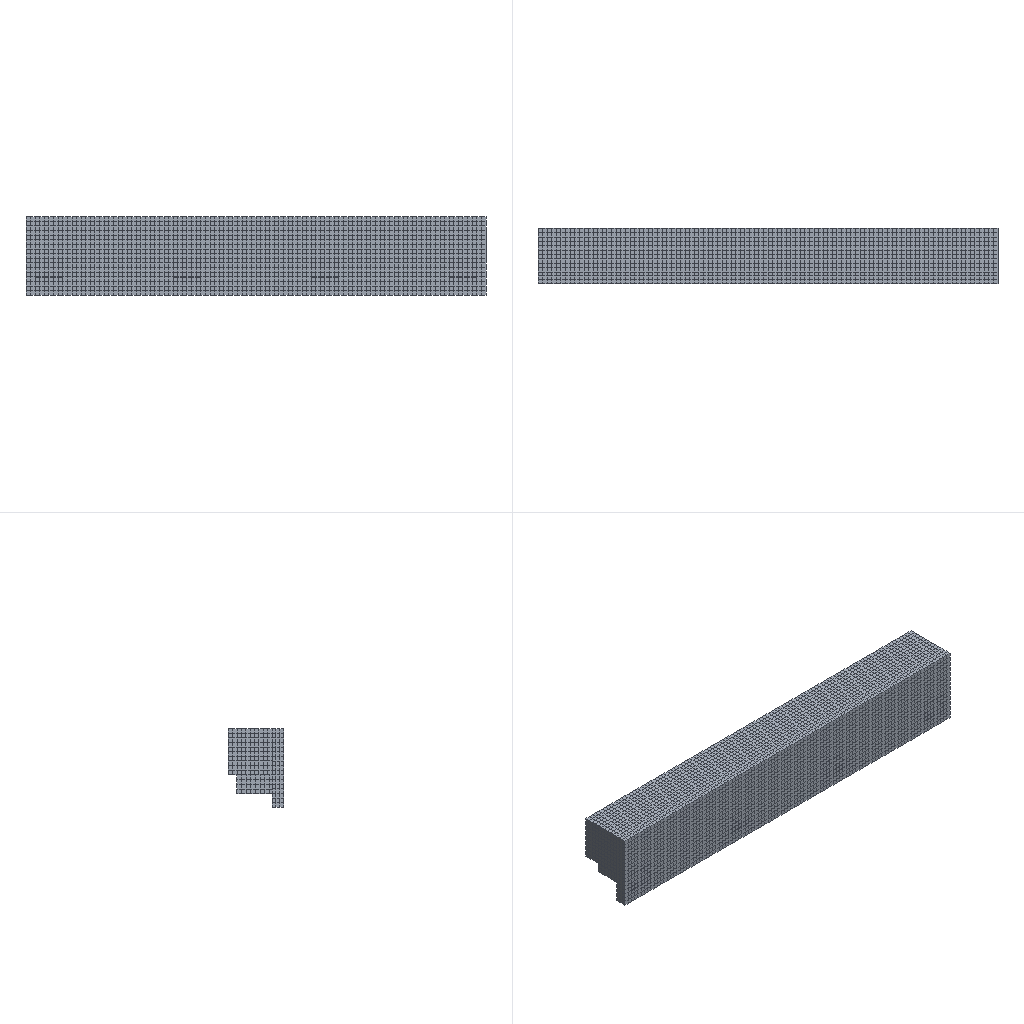Simulation study
Set-up summary:
category,name,step,type,value,unit,region
solver,abaqus
solver,version,,,Abaqus/Explicit 2020
units,not stated in the deck,,not stated
analysis,deck,,transient,transient
load_step,Step-1,Step-1,transient,nlgeom=True
contact,interactions,,,general=1 pairs=0 ties=0
load_step,requested,,,1
mesh,nodes,,,22863
mesh,elements,,,17308
element_type,C3D8R,,solid,17308
load,load commands in deck,,count,1
bc,support commands in deck,,count,6
material,MATERIAL-1,,in results
material,WATER,,in results
check,setup vs results,,match,"per instance, exact: element labels, types and connectivity; labels of the nodes the elements use; coordinates of those nodes at SINGLE_PRECISION in 3 of 3 instance(s)"
Abaqus input file, long lists of numbers shortened:
*Heading
** Job name: Job-1 Model name: Model-1
** Generated by: Abaqus/CAE 2020
*Preprint, echo=NO, model=NO, history=NO, contact=NO
**
** PARTS
**
*Part, name=Part-1
*Node
      1,           2.,           0.,           0.
      2,           4.,           0.,           0.
** (3368 more lines like these left out)
*Element, type=C3D8R
   1,   16,  299,  392,  157,  690,  973, 1066,  831
   2,  529,   95,  472,  502, 1203,  769, 1146, 1176
** (2206 more lines like these left out)
*Nset, nset=Set-1, generate
    1,  3370,     1
*Elset, elset=Set-1, generate
    1,  2208,     1
** Section: Section-1
*Solid Section, elset=Set-1, material=Material-1
,
*End Part
**
*Part, name=water-chong
*Node
      1,           0.,         -9.5,          10.
      2,           0.,  -8.55,          10.
** (12219 more lines like these left out)
*Element, type=C3D8R
    1,   122,   123,   134,   133,     1,     2,    13,    12
    2,   123,   124,   135,   134,     2,     3,    14,    13
** (9998 more lines like these left out)
*Nset, nset=Set-1, generate
     1,  12221,      1
*Elset, elset=Set-1, generate
     1,  10000,      1
** Section: water
*Solid Section, elset=Set-1, controls=EC-1, material=water
,
*End Part
**
*Part, name=water-original
*Node
      1,           0.,         -2.5,   17.1
      2,           0.,  -1.667,   17.1
** (7270 more lines like these left out)
*Element, type=C3D8R
   1,   73,   74,   78,   77,    1,    2,    6,    5
   2,   74,   75,   79,   78,    2,    3,    7,    6
** (5098 more lines like these left out)
*Nset, nset=Set-1, generate
    1,  7272,     1
*Elset, elset=Set-1, generate
    1,  5100,     1
** Section: water
*Solid Section, elset=Set-1, controls=EC-1, material=water
,
*End Part
**
**
** ASSEMBLY
**
*Assembly, name=Assembly
**
*Instance, name=Part-1-1, part=Part-1
*End Instance
**
*Instance, name=water-original-1, part=water-original
         -2.,         -7.7,         -2.9
*End Instance
**
*Instance, name=water-chong-1, part=water-chong
         -2.,          1.8,          4.2
*End Instance
**
*Nset, nset=Set-1, instance=Part-1-1
   47,   48,   49,   61,   62,   63,   75,   76,   77,   89,   90,   91,  217,  218,  219,  220
  243,  244,  245,  246,  269,  270,  271,  272,  295,  296,  297,  298,  721,  722,  723,  735
** (7 more lines like these left out)
*Elset, elset=Set-1, instance=Part-1-1
   74,  119,  121,  133,  152,  159,  197,  246,  247,  248,  249,  257,  258,  259,  260,  269
  270,  271,  272,  273,  283,  284,  285,  286,  626,  671,  673,  685,  704,  711,  749,  798
** (4 more lines like these left out)
*Nset, nset=Set-2, instance=water-original-1, generate
    1,  7269,     4
*Elset, elset=Set-2, instance=water-original-1, generate
    1,  5098,     3
*Nset, nset=Set-3, instance=water-original-1
    1,    2,    3,    4,   69,   70,   71,   72,   73,   74,   75,   76,  141,  142,  143,  144
  145,  146,  147,  148,  213,  214,  215,  216,  217,  218,  219,  220,  285,  286,  287,  288
** (49 more lines like these left out)
*Elset, elset=Set-3, instance=water-original-1
    1,    2,    3,   49,   50,   51,   52,   53,   54,  100,  101,  102,  103,  104,  105,  151
  152,  153,  154,  155,  156,  202,  203,  204,  205,  206,  207,  253,  254,  255,  256,  257
** (36 more lines like these left out)
*Nset, nset=Set-4, instance=water-original-1
    1,    2,    3,    4,    5,    6,    7,    8,    9,   10,   11,   12,   13,   14,   15,   16
   17,   18,   19,   20,   21,   22,   23,   24,   25,   26,   27,   28,   29,   30,   31,   32
** (7 more lines like these left out)
*Elset, elset=Set-4, instance=water-original-1
    1,    2,    3,    4,    5,    6,    7,    8,    9,   10,   11,   12,   13,   14,   15,   16
   17,   18,   19,   20,   21,   22,   23,   24,   25,   26,   27,   28,   29,   30,   31,   32
** (5 more lines like these left out)
*Nset, nset=Set-5, instance=water-chong-1, generate
     1,  12221,      1
*Elset, elset=Set-5, instance=water-chong-1, generate
     1,  10000,      1
*Nset, nset=Set-6, instance=water-chong-1
     1,     2,     3,     4,     5,     6,     7,     8,     9,    10,    11,    12,    13,    14,    15,    16
    17,    18,    19,    20,    21,    22,    23,    24,    25,    26,    27,    28,    29,    30,    31,    32
** (14 more lines like these left out)
*Elset, elset=Set-6, instance=water-chong-1
     1,     2,     3,     4,     5,     6,     7,     8,     9,    10,    11,    12,    13,    14,    15,    16
    17,    18,    19,    20,    21,    22,    23,    24,    25,    26,    27,    28,    29,    30,    31,    32
** (11 more lines like these left out)
*Nset, nset=Set-7, instance=water-chong-1, generate
    11,  12221,     11
*Elset, elset=Set-7, instance=water-chong-1, generate
    10,  10000,     10
*End Assembly
**
** ELEMENT CONTROLS
**
*Section Controls, name=EC-1, ELEMENT CONVERSION=YES, CONVERSION CRITERION=TIME, KERNEL=CUBIC
1., 1., 1.
1, 0.
**
** MATERIALS
**
*Material, name=Material-1
*Damage Initiation, criterion=SHEAR
 0.001,0.,0.
*Damage Evolution, type=DISPLACEMENT
 1e-09,
*Density
2600.,
*Elastic
 2.67e+10, 0.22
*Plastic
 8e+07,0.
*Material, name=water
*Density
1000.,
*Eos, type=USUP
1480.,0.,0.
*Viscosity
 0.01,
**
** INTERACTION PROPERTIES
**
*Surface Interaction, name=IntProp-1
*Friction
 0.2,
*Surface Behavior, pressure-overclosure=HARD
**
** PREDEFINED FIELDS
**
** Name: Predefined Field-1   Type: Velocity
*Initial Conditions, type=VELOCITY
Set-5, 1, 0.
Set-5, 2, 0.
Set-5, 3, -50000.
**
** INTERACTIONS
**
** Interaction: Int-1
*Contact, op=NEW
*Contact Inclusions, ALL EXTERIOR
*Contact Property Assignment
 ,  , IntProp-1
** ----------------------------------------------------------------
**
** STEP: Step-1
**
*Step, name=Step-1, nlgeom=YES
*Dynamic, Explicit
, 0.001
*Bulk Viscosity
0.06, 1.2
** Mass Scaling: Semi-Automatic
**               Whole Model
*Fixed Mass Scaling, factor=500.
**
** BOUNDARY CONDITIONS
**
** Name: BC-1 Type: 对称/反对称/完全固定
*Boundary
Set-1, ENCASTRE
** Name: BC-2 Type: 位移/转角
*Boundary
Set-2, 2, 2
** Name: BC-3 Type: 位移/转角
*Boundary
Set-3, 3, 3
** Name: BC-4 Type: 位移/转角
*Boundary
Set-4, 1, 1
** Name: BC-5 Type: 位移/转角
*Boundary
Set-6, 1, 1
** Name: BC-6 Type: 位移/转角
*Boundary
Set-7, 2, 2
**
** OUTPUT REQUESTS
**
*Restart, write, number interval=1, time marks=NO
**
** FIELD OUTPUT: F-Output-1
**
*Output, field, number interval=50
*Node Output
A, CF, RF, RM, RT, U, V
*Element Output, directions=YES
E, EVF, LE, MISES, MISESONLY, PE, PEEQ, PEEQVAVG, PEVAVG, S, SEQUT, SF, SSAVG, STATUS, SVAVG, YIELDPOT
*Contact Output
CDISP, CSTRESS
**
** HISTORY OUTPUT: H-Output-1
**
*Output, history, variable=PRESELECT
*End Step
Results summary:
result,step,Step-1,completed,increments=33 time=0.001/0.001
result,analysis,,,transient
result,last_loadstep,,,1
result,analysis steps,,count,1
result,primary field,,,U
result,reaction total,,FX,166591600.985,model units
result,reaction total,,FY,-4280214022.758,model units
result,reaction total,,FZ,61234366159.109,model units